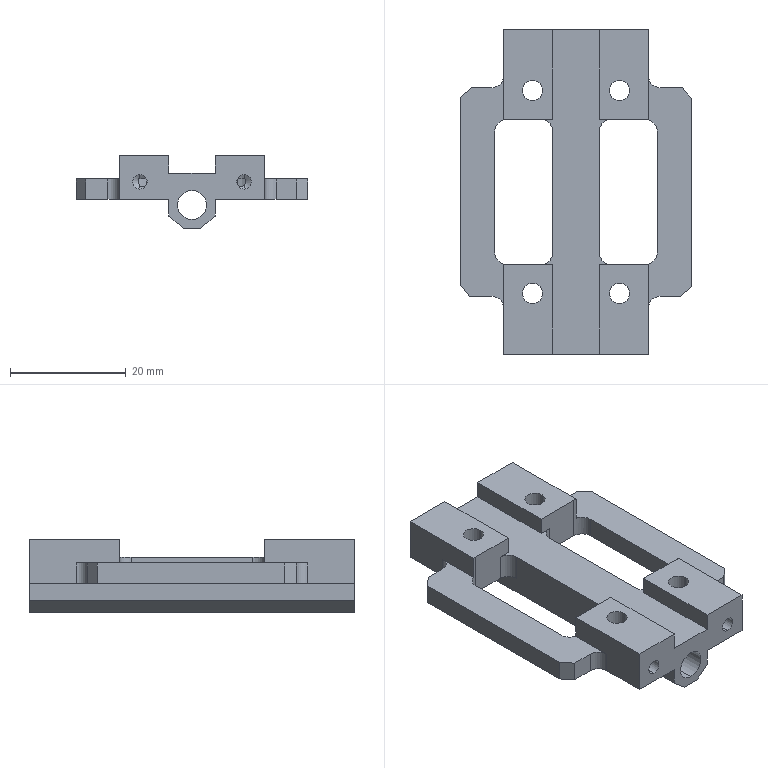Part | SolidWorks | features ICE 7, Chamfer 2, Fillet 2, HoleWzd 2, Extrusion 1 | 1 solid | 90 faces | box 40 x 56 x 12.5 mm | volume 7758 mm3 | plane 44 | cylinder 38 | cone 8 | commonest cylinder face diameters 4 x12 2.5 x8 3.5 x8 6 x8 5 x2